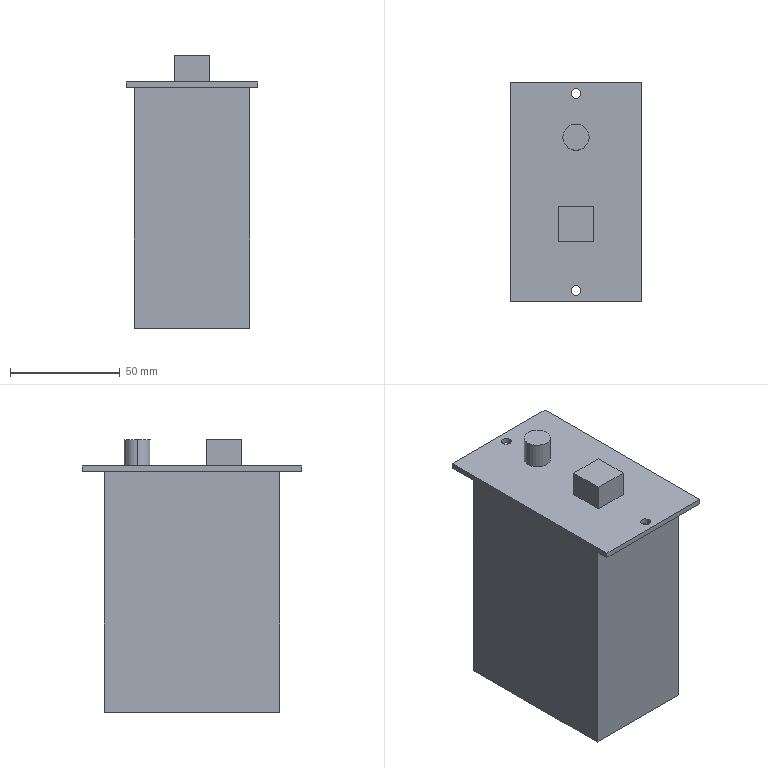Part | STEP file | 1 solid | 23 faces | box 60 x 100 x 124.5 mm | volume 482230 mm3 | plane 17 | cylinder 6 | commonest cylinder face diameters 4.5 x4 12 x2